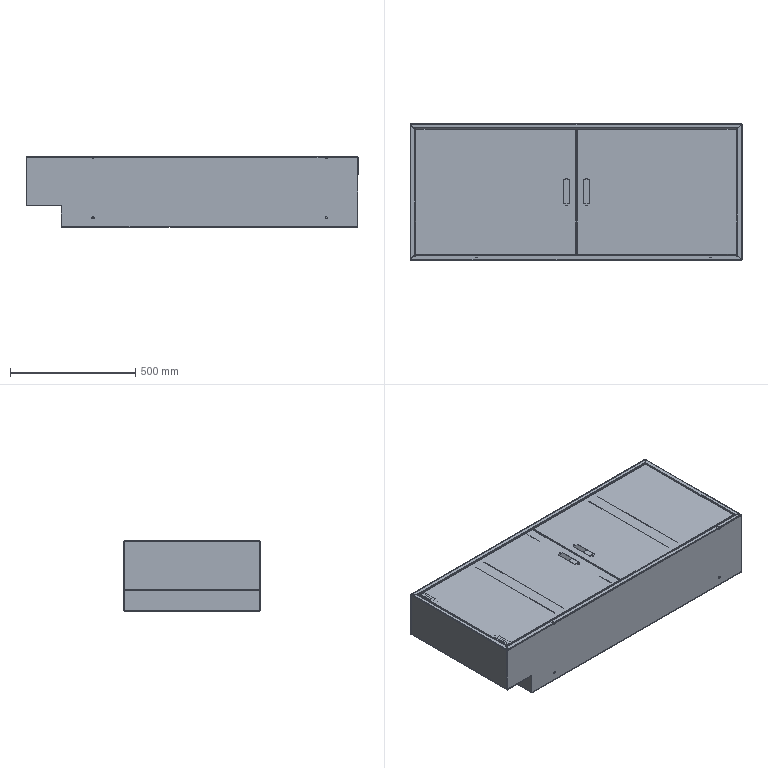Part | SolidWorks | 13 solids | 614 faces | box 1324 x 545 x 280 mm | volume 5555304 mm3 | plane 328 | cylinder 208 | spline 72 | torus 4 | cone 2 | commonest cylinder face diameters 6 x36 1.473 x28 4.473 x28 2 x24 9 x22 5 x16